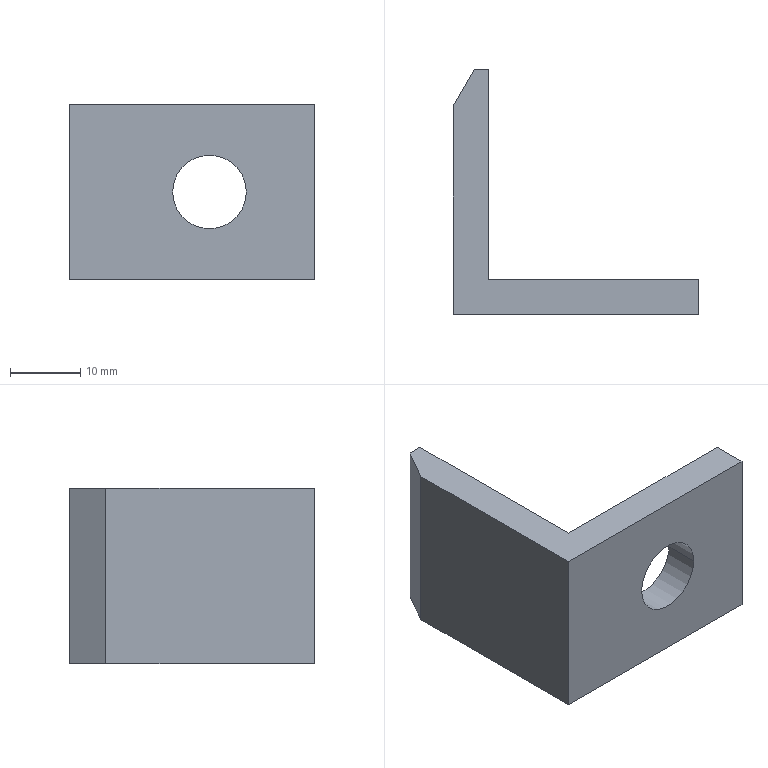Part | STEP file | 44-02-25 Lower Ejector Guide Plate | 1 solid | 11 faces | box 35 x 35 x 25 mm | volume 7497 mm3 | plane 9 | cylinder 2 | commonest cylinder face diameters 10.5 x2
STEP:
#1=CARTESIAN_POINT('',(0.,0.,0.));
#2=DIRECTION('',(0.,0.,1.));
#3=DIRECTION('',(1.,0.,0.));
#4=AXIS2_PLACEMENT_3D('',#1,#2,#3);
#5=CARTESIAN_POINT('',(14.75,0.,0.));
#6=VERTEX_POINT('',#5);
#7=CARTESIAN_POINT('',(14.75,5.,0.));
#8=VERTEX_POINT('',#7);
#9=CARTESIAN_POINT('',(14.75,0.,0.));
#10=DIRECTION('',(0.,1.,0.));
#11=VECTOR('',#10,1.);
#12=LINE('',#9,#11);
#13=CARTESIAN_POINT('',(20.,0.,0.));
#14=DIRECTION('',(0.,1.,0.));
#15=DIRECTION('',(-1.,0.,0.));
#16=AXIS2_PLACEMENT_3D('',#13,#14,#15);
#17=CYLINDRICAL_SURFACE('',#16,5.25);
#18=CARTESIAN_POINT('',(6.283,0.));
#19=DIRECTION('',(0.,1.));
#20=VECTOR('',#19,1.);
#21=LINE('',#18,#20);
#22=(GEOMETRIC_REPRESENTATION_CONTEXT(2)PARAMETRIC_REPRESENTATION_CONTEXT()REPRESENTATION_CONTEXT('',''));
#23=DEFINITIONAL_REPRESENTATION('',(#21),#22);
#24=PCURVE('',#17,#23);
#25=CARTESIAN_POINT('',(20.,0.,0.));
#26=DIRECTION('',(0.,1.,0.));
#27=DIRECTION('',(-1.,0.,0.));
#28=AXIS2_PLACEMENT_3D('',#25,#26,#27);
#29=CYLINDRICAL_SURFACE('',#28,5.25);
#30=CARTESIAN_POINT('',(0.,0.));
#31=DIRECTION('',(0.,1.));
#32=VECTOR('',#31,1.);
#33=LINE('',#30,#32);
#34=(GEOMETRIC_REPRESENTATION_CONTEXT(2)PARAMETRIC_REPRESENTATION_CONTEXT()REPRESENTATION_CONTEXT('',''));
#35=DEFINITIONAL_REPRESENTATION('',(#33),#34);
#36=PCURVE('',#29,#35);
#37=SURFACE_CURVE('',#12,(#24,#36),.PCURVE_S1.);
#38=EDGE_CURVE('',#6,#8,#37,.T.);
#39=ORIENTED_EDGE('',*,*,#38,.T.);
#40=CARTESIAN_POINT('',(25.25,5.,0.));
#41=VERTEX_POINT('',#40);
#42=CARTESIAN_POINT('',(20.,5.,0.));
#43=DIRECTION('',(0.,1.,0.));
#44=DIRECTION('',(-1.,0.,0.));
#45=AXIS2_PLACEMENT_3D('',#42,#43,#44);
#46=CIRCLE('',#45,5.25);
#47=CARTESIAN_POINT('',(0.,5.));
#48=DIRECTION('',(1.,0.));
#49=VECTOR('',#48,1.);
#50=LINE('',#47,#49);
#51=(GEOMETRIC_REPRESENTATION_CONTEXT(2)PARAMETRIC_REPRESENTATION_CONTEXT()REPRESENTATION_CONTEXT('',''));
#52=DEFINITIONAL_REPRESENTATION('',(#50),#51);
#53=PCURVE('',#17,#52);
#54=CARTESIAN_POINT('',(35.,5.,12.5));
#55=DIRECTION('',(0.,-1.,0.));
#56=DIRECTION('',(1.,0.,0.));
#57=AXIS2_PLACEMENT_3D('',#54,#55,#56);
#58=PLANE('',#57);
#59=CARTESIAN_POINT('',(-20.25,-12.5));
#60=CARTESIAN_POINT('',(-20.25,-3.407));
#61=CARTESIAN_POINT('',(-12.375,-7.953));
#62=CARTESIAN_POINT('',(-4.5,-12.5));
#63=CARTESIAN_POINT('',(-12.375,-17.047));
#64=CARTESIAN_POINT('',(-20.25,-21.593));
#65=CARTESIAN_POINT('',(-20.25,-12.5));
#66=(BOUNDED_CURVE()B_SPLINE_CURVE(2,(#59,#60,#61,#62,#63,#64,#65),.UNSPECIFIED.,.T.,.F.)B_SPLINE_CURVE_WITH_KNOTS((1,2,2,2,2,1),(-2.094,0.,2.094,4.189,6.283,8.378),.UNSPECIFIED.)CURVE()GEOMETRIC_REPRESENTATION_ITEM()RATIONAL_B_SPLINE_CURVE((1.,0.5,1.,0.5,1.,0.5,1.))REPRESENTATION_ITEM(''));
#67=(GEOMETRIC_REPRESENTATION_CONTEXT(2)PARAMETRIC_REPRESENTATION_CONTEXT()REPRESENTATION_CONTEXT('',''));
#68=DEFINITIONAL_REPRESENTATION('',(#66),#67);
#69=PCURVE('',#58,#68);
#70=SURFACE_CURVE('',#46,(#53,#69),.PCURVE_S1.);
#71=EDGE_CURVE('',#41,#8,#70,.T.);
#72=ORIENTED_EDGE('',*,*,#71,.F.);
#73=CARTESIAN_POINT('',(25.25,0.,0.));
#74=VERTEX_POINT('',#73);
#75=CARTESIAN_POINT('',(25.25,0.,0.));
#76=DIRECTION('',(0.,1.,0.));
#77=VECTOR('',#76,1.);
#78=LINE('',#75,#77);
#79=CARTESIAN_POINT('',(3.142,0.));
#80=DIRECTION('',(0.,1.));
#81=VECTOR('',#80,1.);
#82=LINE('',#79,#81);
#83=(GEOMETRIC_REPRESENTATION_CONTEXT(2)PARAMETRIC_REPRESENTATION_CONTEXT()REPRESENTATION_CONTEXT('',''));
#84=DEFINITIONAL_REPRESENTATION('',(#82),#83);
#85=PCURVE('',#17,#84);
#86=CARTESIAN_POINT('',(3.142,0.));
#87=DIRECTION('',(0.,1.));
#88=VECTOR('',#87,1.);
#89=LINE('',#86,#88);
#90=(GEOMETRIC_REPRESENTATION_CONTEXT(2)PARAMETRIC_REPRESENTATION_CONTEXT()REPRESENTATION_CONTEXT('',''));
#91=DEFINITIONAL_REPRESENTATION('',(#89),#90);
#92=PCURVE('',#29,#91);
#93=SURFACE_CURVE('',#78,(#85,#92),.PCURVE_S1.);
#94=EDGE_CURVE('',#74,#41,#93,.T.);
#95=ORIENTED_EDGE('',*,*,#94,.F.);
#96=CARTESIAN_POINT('',(20.,0.,0.));
#97=DIRECTION('',(0.,1.,0.));
#98=DIRECTION('',(-1.,0.,0.));
#99=AXIS2_PLACEMENT_3D('',#96,#97,#98);
#100=CIRCLE('',#99,5.25);
#101=CARTESIAN_POINT('',(0.,0.));
#102=DIRECTION('',(1.,0.));
#103=VECTOR('',#102,1.);
#104=LINE('',#101,#103);
#105=(GEOMETRIC_REPRESENTATION_CONTEXT(2)PARAMETRIC_REPRESENTATION_CONTEXT()REPRESENTATION_CONTEXT('',''));
#106=DEFINITIONAL_REPRESENTATION('',(#104),#105);
#107=PCURVE('',#17,#106);
#108=CARTESIAN_POINT('',(0.,0.,12.5));
#109=DIRECTION('',(0.,1.,0.));
#110=DIRECTION('',(0.,0.,1.));
#111=AXIS2_PLACEMENT_3D('',#108,#109,#110);
#112=PLANE('',#111);
#113=CARTESIAN_POINT('',(-12.5,20.));
#114=DIRECTION('',(0.,-1.));
#115=AXIS2_PLACEMENT_2D('',#113,#114);
#116=CIRCLE('',#115,5.25);
#117=(GEOMETRIC_REPRESENTATION_CONTEXT(2)PARAMETRIC_REPRESENTATION_CONTEXT()REPRESENTATION_CONTEXT('',''));
#118=DEFINITIONAL_REPRESENTATION('',(#116),#117);
#119=PCURVE('',#112,#118);
#120=SURFACE_CURVE('',#100,(#107,#119),.PCURVE_S1.);
#121=EDGE_CURVE('',#74,#6,#120,.T.);
#122=ORIENTED_EDGE('',*,*,#121,.T.);
#123=EDGE_LOOP('',(#39,#72,#95,#122));
#124=FACE_BOUND('',#123,.F.);
#125=ADVANCED_FACE('',(#124),#17,.F.);
#126=CARTESIAN_POINT('',(5.,35.,-12.5));
#127=VERTEX_POINT('',#126);
#128=CARTESIAN_POINT('',(3.,35.,-12.5));
#129=VERTEX_POINT('',#128);
#130=CARTESIAN_POINT('',(5.,35.,-12.5));
#131=DIRECTION('',(-1.,0.,0.));
#132=VECTOR('',#131,1.);
#133=LINE('',#130,#132);
#134=CARTESIAN_POINT('',(5.,35.,12.5));
#135=DIRECTION('',(0.,-1.,0.));
#136=DIRECTION('',(0.,0.,-1.));
#137=AXIS2_PLACEMENT_3D('',#134,#135,#136);
#138=PLANE('',#137);
#139=CARTESIAN_POINT('',(25.,0.));
#140=DIRECTION('',(0.,-1.));
#141=VECTOR('',#140,1.);
#142=LINE('',#139,#141);
#143=(GEOMETRIC_REPRESENTATION_CONTEXT(2)PARAMETRIC_REPRESENTATION_CONTEXT()REPRESENTATION_CONTEXT('',''));
#144=DEFINITIONAL_REPRESENTATION('',(#142),#143);
#145=PCURVE('',#138,#144);
#146=CARTESIAN_POINT('',(0.,0.,-12.5));
#147=DIRECTION('',(0.,0.,1.));
#148=DIRECTION('',(1.,0.,0.));
#149=AXIS2_PLACEMENT_3D('',#146,#147,#148);
#150=PLANE('',#149);
#151=CARTESIAN_POINT('',(5.,35.));
#152=DIRECTION('',(-1.,0.));
#153=VECTOR('',#152,1.);
#154=LINE('',#151,#153);
#155=(GEOMETRIC_REPRESENTATION_CONTEXT(2)PARAMETRIC_REPRESENTATION_CONTEXT()REPRESENTATION_CONTEXT('',''));
#156=DEFINITIONAL_REPRESENTATION('',(#154),#155);
#157=PCURVE('',#150,#156);
#158=SURFACE_CURVE('',#133,(#145,#157),.PCURVE_S1.);
#159=EDGE_CURVE('',#127,#129,#158,.T.);
#160=ORIENTED_EDGE('',*,*,#159,.T.);
#161=CARTESIAN_POINT('',(3.,35.,12.5));
#162=VERTEX_POINT('',#161);
#163=CARTESIAN_POINT('',(3.,35.,12.5));
#164=DIRECTION('',(0.,0.,1.));
#165=VECTOR('',#164,1.);
#166=LINE('',#163,#165);
#167=CARTESIAN_POINT('',(0.,-2.));
#168=DIRECTION('',(-1.,0.));
#169=VECTOR('',#168,1.);
#170=LINE('',#167,#169);
#171=(GEOMETRIC_REPRESENTATION_CONTEXT(2)PARAMETRIC_REPRESENTATION_CONTEXT()REPRESENTATION_CONTEXT('',''));
#172=DEFINITIONAL_REPRESENTATION('',(#170),#171);
#173=PCURVE('',#138,#172);
#174=CARTESIAN_POINT('',(0.,29.804,12.5));
#175=DIRECTION('',(0.866,-0.5,0.));
#176=DIRECTION('',(0.,0.,-1.));
#177=AXIS2_PLACEMENT_3D('',#174,#175,#176);
#178=PLANE('',#177);
#179=CARTESIAN_POINT('',(0.,6.));
#180=DIRECTION('',(-1.,0.));
#181=VECTOR('',#180,1.);
#182=LINE('',#179,#181);
#183=(GEOMETRIC_REPRESENTATION_CONTEXT(2)PARAMETRIC_REPRESENTATION_CONTEXT()REPRESENTATION_CONTEXT('',''));
#184=DEFINITIONAL_REPRESENTATION('',(#182),#183);
#185=PCURVE('',#178,#184);
#186=SURFACE_CURVE('',#166,(#173,#185),.PCURVE_S1.);
#187=EDGE_CURVE('',#129,#162,#186,.T.);
#188=ORIENTED_EDGE('',*,*,#187,.T.);
#189=CARTESIAN_POINT('',(5.,35.,12.5));
#190=VERTEX_POINT('',#189);
#191=CARTESIAN_POINT('',(5.,35.,12.5));
#192=DIRECTION('',(-1.,0.,0.));
#193=VECTOR('',#192,1.);
#194=LINE('',#191,#193);
#195=CARTESIAN_POINT('',(0.,0.));
#196=DIRECTION('',(0.,-1.));
#197=VECTOR('',#196,1.);
#198=LINE('',#195,#197);
#199=(GEOMETRIC_REPRESENTATION_CONTEXT(2)PARAMETRIC_REPRESENTATION_CONTEXT()REPRESENTATION_CONTEXT('',''));
#200=DEFINITIONAL_REPRESENTATION('',(#198),#199);
#201=PCURVE('',#138,#200);
#202=CARTESIAN_POINT('',(0.,0.,12.5));
#203=DIRECTION('',(0.,0.,1.));
#204=DIRECTION('',(1.,0.,0.));
#205=AXIS2_PLACEMENT_3D('',#202,#203,#204);
#206=PLANE('',#205);
#207=CARTESIAN_POINT('',(5.,35.));
#208=DIRECTION('',(-1.,0.));
#209=VECTOR('',#208,1.);
#210=LINE('',#207,#209);
#211=(GEOMETRIC_REPRESENTATION_CONTEXT(2)PARAMETRIC_REPRESENTATION_CONTEXT()REPRESENTATION_CONTEXT('',''));
#212=DEFINITIONAL_REPRESENTATION('',(#210),#211);
#213=PCURVE('',#206,#212);
#214=SURFACE_CURVE('',#194,(#201,#213),.PCURVE_S1.);
#215=EDGE_CURVE('',#190,#162,#214,.T.);
#216=ORIENTED_EDGE('',*,*,#215,.F.);
#217=CARTESIAN_POINT('',(5.,35.,12.5));
#218=DIRECTION('',(0.,0.,-1.));
#219=VECTOR('',#218,1.);
#220=LINE('',#217,#219);
#221=CARTESIAN_POINT('',(0.,0.));
#222=DIRECTION('',(1.,0.));
#223=VECTOR('',#222,1.);
#224=LINE('',#221,#223);
#225=(GEOMETRIC_REPRESENTATION_CONTEXT(2)PARAMETRIC_REPRESENTATION_CONTEXT()REPRESENTATION_CONTEXT('',''));
#226=DEFINITIONAL_REPRESENTATION('',(#224),#225);
#227=PCURVE('',#138,#226);
#228=CARTESIAN_POINT('',(5.,5.,12.5));
#229=DIRECTION('',(-1.,0.,0.));
#230=DIRECTION('',(0.,-1.,0.));
#231=AXIS2_PLACEMENT_3D('',#228,#229,#230);
#232=PLANE('',#231);
#233=CARTESIAN_POINT('',(-30.,0.));
#234=DIRECTION('',(0.,-1.));
#235=VECTOR('',#234,1.);
#236=LINE('',#233,#235);
#237=(GEOMETRIC_REPRESENTATION_CONTEXT(2)PARAMETRIC_REPRESENTATION_CONTEXT()REPRESENTATION_CONTEXT('',''));
#238=DEFINITIONAL_REPRESENTATION('',(#236),#237);
#239=PCURVE('',#232,#238);
#240=SURFACE_CURVE('',#220,(#227,#239),.PCURVE_S1.);
#241=EDGE_CURVE('',#190,#127,#240,.T.);
#242=ORIENTED_EDGE('',*,*,#241,.T.);
#243=EDGE_LOOP('',(#160,#188,#216,#242));
#244=FACE_BOUND('',#243,.T.);
#245=ADVANCED_FACE('',(#244),#138,.F.);
#246=CARTESIAN_POINT('',(0.,29.804,12.5));
#247=VERTEX_POINT('',#246);
#248=CARTESIAN_POINT('',(0.,0.,12.5));
#249=VERTEX_POINT('',#248);
#250=CARTESIAN_POINT('',(0.,35.,12.5));
#251=DIRECTION('',(0.,-1.,0.));
#252=VECTOR('',#251,1.);
#253=LINE('',#250,#252);
#254=CARTESIAN_POINT('',(0.,35.,12.5));
#255=DIRECTION('',(1.,0.,0.));
#256=DIRECTION('',(0.,0.,-1.));
#257=AXIS2_PLACEMENT_3D('',#254,#255,#256);
#258=PLANE('',#257);
#259=CARTESIAN_POINT('',(0.,0.));
#260=DIRECTION('',(0.,-1.));
#261=VECTOR('',#260,1.);
#262=LINE('',#259,#261);
#263=(GEOMETRIC_REPRESENTATION_CONTEXT(2)PARAMETRIC_REPRESENTATION_CONTEXT()REPRESENTATION_CONTEXT('',''));
#264=DEFINITIONAL_REPRESENTATION('',(#262),#263);
#265=PCURVE('',#258,#264);
#266=CARTESIAN_POINT('',(0.,35.));
#267=DIRECTION('',(0.,-1.));
#268=VECTOR('',#267,1.);
#269=LINE('',#266,#268);
#270=(GEOMETRIC_REPRESENTATION_CONTEXT(2)PARAMETRIC_REPRESENTATION_CONTEXT()REPRESENTATION_CONTEXT('',''));
#271=DEFINITIONAL_REPRESENTATION('',(#269),#270);
#272=PCURVE('',#206,#271);
#273=SURFACE_CURVE('',#253,(#265,#272),.PCURVE_S1.);
#274=EDGE_CURVE('',#247,#249,#273,.T.);
#275=ORIENTED_EDGE('',*,*,#274,.F.);
#276=CARTESIAN_POINT('',(0.,29.804,-12.5));
#277=VERTEX_POINT('',#276);
#278=CARTESIAN_POINT('',(0.,29.804,12.5));
#279=DIRECTION('',(0.,0.,-1.));
#280=VECTOR('',#279,1.);
#281=LINE('',#278,#280);
#282=CARTESIAN_POINT('',(0.,-5.196));
#283=DIRECTION('',(1.,0.));
#284=VECTOR('',#283,1.);
#285=LINE('',#282,#284);
#286=(GEOMETRIC_REPRESENTATION_CONTEXT(2)PARAMETRIC_REPRESENTATION_CONTEXT()REPRESENTATION_CONTEXT('',''));
#287=DEFINITIONAL_REPRESENTATION('',(#285),#286);
#288=PCURVE('',#258,#287);
#289=CARTESIAN_POINT('',(0.,0.));
#290=DIRECTION('',(1.,0.));
#291=VECTOR('',#290,1.);
#292=LINE('',#289,#291);
#293=(GEOMETRIC_REPRESENTATION_CONTEXT(2)PARAMETRIC_REPRESENTATION_CONTEXT()REPRESENTATION_CONTEXT('',''));
#294=DEFINITIONAL_REPRESENTATION('',(#292),#293);
#295=PCURVE('',#178,#294);
#296=SURFACE_CURVE('',#281,(#288,#295),.PCURVE_S1.);
#297=EDGE_CURVE('',#247,#277,#296,.T.);
#298=ORIENTED_EDGE('',*,*,#297,.T.);
#299=CARTESIAN_POINT('',(0.,0.,-12.5));
#300=VERTEX_POINT('',#299);
#301=CARTESIAN_POINT('',(0.,35.,-12.5));
#302=DIRECTION('',(0.,-1.,0.));
#303=VECTOR('',#302,1.);
#304=LINE('',#301,#303);
#305=CARTESIAN_POINT('',(25.,0.));
#306=DIRECTION('',(0.,-1.));
#307=VECTOR('',#306,1.);
#308=LINE('',#305,#307);
#309=(GEOMETRIC_REPRESENTATION_CONTEXT(2)PARAMETRIC_REPRESENTATION_CONTEXT()REPRESENTATION_CONTEXT('',''));
#310=DEFINITIONAL_REPRESENTATION('',(#308),#309);
#311=PCURVE('',#258,#310);
#312=CARTESIAN_POINT('',(0.,35.));
#313=DIRECTION('',(0.,-1.));
#314=VECTOR('',#313,1.);
#315=LINE('',#312,#314);
#316=(GEOMETRIC_REPRESENTATION_CONTEXT(2)PARAMETRIC_REPRESENTATION_CONTEXT()REPRESENTATION_CONTEXT('',''));
#317=DEFINITIONAL_REPRESENTATION('',(#315),#316);
#318=PCURVE('',#150,#317);
#319=SURFACE_CURVE('',#304,(#311,#318),.PCURVE_S1.);
#320=EDGE_CURVE('',#277,#300,#319,.T.);
#321=ORIENTED_EDGE('',*,*,#320,.T.);
#322=CARTESIAN_POINT('',(0.,0.,12.5));
#323=DIRECTION('',(0.,0.,-1.));
#324=VECTOR('',#323,1.);
#325=LINE('',#322,#324);
#326=CARTESIAN_POINT('',(0.,-35.));
#327=DIRECTION('',(1.,0.));
#328=VECTOR('',#327,1.);
#329=LINE('',#326,#328);
#330=(GEOMETRIC_REPRESENTATION_CONTEXT(2)PARAMETRIC_REPRESENTATION_CONTEXT()REPRESENTATION_CONTEXT('',''));
#331=DEFINITIONAL_REPRESENTATION('',(#329),#330);
#332=PCURVE('',#258,#331);
#333=CARTESIAN_POINT('',(0.,0.));
#334=DIRECTION('',(-1.,0.));
#335=VECTOR('',#334,1.);
#336=LINE('',#333,#335);
#337=(GEOMETRIC_REPRESENTATION_CONTEXT(2)PARAMETRIC_REPRESENTATION_CONTEXT()REPRESENTATION_CONTEXT('',''));
#338=DEFINITIONAL_REPRESENTATION('',(#336),#337);
#339=PCURVE('',#112,#338);
#340=SURFACE_CURVE('',#325,(#332,#339),.PCURVE_S1.);
#341=EDGE_CURVE('',#249,#300,#340,.T.);
#342=ORIENTED_EDGE('',*,*,#341,.F.);
#343=EDGE_LOOP('',(#275,#298,#321,#342));
#344=FACE_BOUND('',#343,.T.);
#345=ADVANCED_FACE('',(#344),#258,.F.);
#346=CARTESIAN_POINT('',(20.,0.,0.));
#347=DIRECTION('',(0.,1.,0.));
#348=DIRECTION('',(-1.,0.,0.));
#349=AXIS2_PLACEMENT_3D('',#346,#347,#348);
#350=CIRCLE('',#349,5.25);
#351=CARTESIAN_POINT('',(-12.5,20.));
#352=DIRECTION('',(0.,-1.));
#353=AXIS2_PLACEMENT_2D('',#351,#352);
#354=CIRCLE('',#353,5.25);
#355=(GEOMETRIC_REPRESENTATION_CONTEXT(2)PARAMETRIC_REPRESENTATION_CONTEXT()REPRESENTATION_CONTEXT('',''));
#356=DEFINITIONAL_REPRESENTATION('',(#354),#355);
#357=PCURVE('',#112,#356);
#358=CARTESIAN_POINT('',(0.,0.));
#359=DIRECTION('',(1.,0.));
#360=VECTOR('',#359,1.);
#361=LINE('',#358,#360);
#362=(GEOMETRIC_REPRESENTATION_CONTEXT(2)PARAMETRIC_REPRESENTATION_CONTEXT()REPRESENTATION_CONTEXT('',''));
#363=DEFINITIONAL_REPRESENTATION('',(#361),#362);
#364=PCURVE('',#29,#363);
#365=SURFACE_CURVE('',#350,(#357,#364),.PCURVE_S1.);
#366=EDGE_CURVE('',#6,#74,#365,.T.);
#367=ORIENTED_EDGE('',*,*,#366,.T.);
#368=ORIENTED_EDGE('',*,*,#121,.T.);
#369=EDGE_LOOP('',(#367,#368));
#370=FACE_BOUND('',#369,.T.);
#371=CARTESIAN_POINT('',(35.,0.,-12.5));
#372=VERTEX_POINT('',#371);
#373=CARTESIAN_POINT('',(0.,0.,-12.5));
#374=DIRECTION('',(1.,0.,0.));
#375=VECTOR('',#374,1.);
#376=LINE('',#373,#375);
#377=CARTESIAN_POINT('',(-25.,0.));
#378=DIRECTION('',(0.,1.));
#379=VECTOR('',#378,1.);
#380=LINE('',#377,#379);
#381=(GEOMETRIC_REPRESENTATION_CONTEXT(2)PARAMETRIC_REPRESENTATION_CONTEXT()REPRESENTATION_CONTEXT('',''));
#382=DEFINITIONAL_REPRESENTATION('',(#380),#381);
#383=PCURVE('',#112,#382);
#384=CARTESIAN_POINT('',(0.,0.));
#385=DIRECTION('',(1.,0.));
#386=VECTOR('',#385,1.);
#387=LINE('',#384,#386);
#388=(GEOMETRIC_REPRESENTATION_CONTEXT(2)PARAMETRIC_REPRESENTATION_CONTEXT()REPRESENTATION_CONTEXT('',''));
#389=DEFINITIONAL_REPRESENTATION('',(#387),#388);
#390=PCURVE('',#150,#389);
#391=SURFACE_CURVE('',#376,(#383,#390),.PCURVE_S1.);
#392=EDGE_CURVE('',#300,#372,#391,.T.);
#393=ORIENTED_EDGE('',*,*,#392,.T.);
#394=CARTESIAN_POINT('',(35.,0.,12.5));
#395=VERTEX_POINT('',#394);
#396=CARTESIAN_POINT('',(35.,0.,12.5));
#397=DIRECTION('',(0.,0.,-1.));
#398=VECTOR('',#397,1.);
#399=LINE('',#396,#398);
#400=CARTESIAN_POINT('',(0.,35.));
#401=DIRECTION('',(-1.,0.));
#402=VECTOR('',#401,1.);
#403=LINE('',#400,#402);
#404=(GEOMETRIC_REPRESENTATION_CONTEXT(2)PARAMETRIC_REPRESENTATION_CONTEXT()REPRESENTATION_CONTEXT('',''));
#405=DEFINITIONAL_REPRESENTATION('',(#403),#404);
#406=PCURVE('',#112,#405);
#407=CARTESIAN_POINT('',(35.,0.,12.5));
#408=DIRECTION('',(-1.,0.,0.));
#409=DIRECTION('',(0.,0.,1.));
#410=AXIS2_PLACEMENT_3D('',#407,#408,#409);
#411=PLANE('',#410);
#412=CARTESIAN_POINT('',(0.,0.));
#413=DIRECTION('',(-1.,0.));
#414=VECTOR('',#413,1.);
#415=LINE('',#412,#414);
#416=(GEOMETRIC_REPRESENTATION_CONTEXT(2)PARAMETRIC_REPRESENTATION_CONTEXT()REPRESENTATION_CONTEXT('',''));
#417=DEFINITIONAL_REPRESENTATION('',(#415),#416);
#418=PCURVE('',#411,#417);
#419=SURFACE_CURVE('',#399,(#406,#418),.PCURVE_S1.);
#420=EDGE_CURVE('',#395,#372,#419,.T.);
#421=ORIENTED_EDGE('',*,*,#420,.F.);
#422=CARTESIAN_POINT('',(0.,0.,12.5));
#423=DIRECTION('',(1.,0.,0.));
#424=VECTOR('',#423,1.);
#425=LINE('',#422,#424);
#426=CARTESIAN_POINT('',(0.,0.));
#427=DIRECTION('',(0.,1.));
#428=VECTOR('',#427,1.);
#429=LINE('',#426,#428);
#430=(GEOMETRIC_REPRESENTATION_CONTEXT(2)PARAMETRIC_REPRESENTATION_CONTEXT()REPRESENTATION_CONTEXT('',''));
#431=DEFINITIONAL_REPRESENTATION('',(#429),#430);
#432=PCURVE('',#112,#431);
#433=CARTESIAN_POINT('',(0.,0.));
#434=DIRECTION('',(1.,0.));
#435=VECTOR('',#434,1.);
#436=LINE('',#433,#435);
#437=(GEOMETRIC_REPRESENTATION_CONTEXT(2)PARAMETRIC_REPRESENTATION_CONTEXT()REPRESENTATION_CONTEXT('',''));
#438=DEFINITIONAL_REPRESENTATION('',(#436),#437);
#439=PCURVE('',#206,#438);
#440=SURFACE_CURVE('',#425,(#432,#439),.PCURVE_S1.);
#441=EDGE_CURVE('',#249,#395,#440,.T.);
#442=ORIENTED_EDGE('',*,*,#441,.F.);
#443=ORIENTED_EDGE('',*,*,#341,.T.);
#444=EDGE_LOOP('',(#393,#421,#442,#443));
#445=FACE_BOUND('',#444,.T.);
#446=ADVANCED_FACE('',(#370,#445),#112,.F.);
#447=CARTESIAN_POINT('',(35.,5.,-12.5));
#448=VERTEX_POINT('',#447);
#449=CARTESIAN_POINT('',(35.,0.,-12.5));
#450=DIRECTION('',(0.,1.,0.));
#451=VECTOR('',#450,1.);
#452=LINE('',#449,#451);
#453=CARTESIAN_POINT('',(-25.,0.));
#454=DIRECTION('',(0.,1.));
#455=VECTOR('',#454,1.);
#456=LINE('',#453,#455);
#457=(GEOMETRIC_REPRESENTATION_CONTEXT(2)PARAMETRIC_REPRESENTATION_CONTEXT()REPRESENTATION_CONTEXT('',''));
#458=DEFINITIONAL_REPRESENTATION('',(#456),#457);
#459=PCURVE('',#411,#458);
#460=CARTESIAN_POINT('',(35.,0.));
#461=DIRECTION('',(0.,1.));
#462=VECTOR('',#461,1.);
#463=LINE('',#460,#462);
#464=(GEOMETRIC_REPRESENTATION_CONTEXT(2)PARAMETRIC_REPRESENTATION_CONTEXT()REPRESENTATION_CONTEXT('',''));
#465=DEFINITIONAL_REPRESENTATION('',(#463),#464);
#466=PCURVE('',#150,#465);
#467=SURFACE_CURVE('',#452,(#459,#466),.PCURVE_S1.);
#468=EDGE_CURVE('',#372,#448,#467,.T.);
#469=ORIENTED_EDGE('',*,*,#468,.T.);
#470=CARTESIAN_POINT('',(35.,5.,12.5));
#471=VERTEX_POINT('',#470);
#472=CARTESIAN_POINT('',(35.,5.,12.5));
#473=DIRECTION('',(0.,0.,-1.));
#474=VECTOR('',#473,1.);
#475=LINE('',#472,#474);
#476=CARTESIAN_POINT('',(0.,5.));
#477=DIRECTION('',(-1.,0.));
#478=VECTOR('',#477,1.);
#479=LINE('',#476,#478);
#480=(GEOMETRIC_REPRESENTATION_CONTEXT(2)PARAMETRIC_REPRESENTATION_CONTEXT()REPRESENTATION_CONTEXT('',''));
#481=DEFINITIONAL_REPRESENTATION('',(#479),#480);
#482=PCURVE('',#411,#481);
#483=CARTESIAN_POINT('',(0.,0.));
#484=DIRECTION('',(0.,-1.));
#485=VECTOR('',#484,1.);
#486=LINE('',#483,#485);
#487=(GEOMETRIC_REPRESENTATION_CONTEXT(2)PARAMETRIC_REPRESENTATION_CONTEXT()REPRESENTATION_CONTEXT('',''));
#488=DEFINITIONAL_REPRESENTATION('',(#486),#487);
#489=PCURVE('',#58,#488);
#490=SURFACE_CURVE('',#475,(#482,#489),.PCURVE_S1.);
#491=EDGE_CURVE('',#471,#448,#490,.T.);
#492=ORIENTED_EDGE('',*,*,#491,.F.);
#493=CARTESIAN_POINT('',(35.,0.,12.5));
#494=DIRECTION('',(0.,1.,0.));
#495=VECTOR('',#494,1.);
#496=LINE('',#493,#495);
#497=CARTESIAN_POINT('',(0.,0.));
#498=DIRECTION('',(0.,1.));
#499=VECTOR('',#498,1.);
#500=LINE('',#497,#499);
#501=(GEOMETRIC_REPRESENTATION_CONTEXT(2)PARAMETRIC_REPRESENTATION_CONTEXT()REPRESENTATION_CONTEXT('',''));
#502=DEFINITIONAL_REPRESENTATION('',(#500),#501);
#503=PCURVE('',#411,#502);
#504=CARTESIAN_POINT('',(35.,0.));
#505=DIRECTION('',(0.,1.));
#506=VECTOR('',#505,1.);
#507=LINE('',#504,#506);
#508=(GEOMETRIC_REPRESENTATION_CONTEXT(2)PARAMETRIC_REPRESENTATION_CONTEXT()REPRESENTATION_CONTEXT('',''));
#509=DEFINITIONAL_REPRESENTATION('',(#507),#508);
#510=PCURVE('',#206,#509);
#511=SURFACE_CURVE('',#496,(#503,#510),.PCURVE_S1.);
#512=EDGE_CURVE('',#395,#471,#511,.T.);
#513=ORIENTED_EDGE('',*,*,#512,.F.);
#514=ORIENTED_EDGE('',*,*,#420,.T.);
#515=EDGE_LOOP('',(#469,#492,#513,#514));
#516=FACE_BOUND('',#515,.T.);
#517=ADVANCED_FACE('',(#516),#411,.F.);
#518=CARTESIAN_POINT('',(20.,5.,0.));
#519=DIRECTION('',(0.,1.,0.));
#520=DIRECTION('',(-1.,0.,0.));
#521=AXIS2_PLACEMENT_3D('',#518,#519,#520);
#522=CIRCLE('',#521,5.25);
#523=CARTESIAN_POINT('',(-20.25,-12.5));
#524=CARTESIAN_POINT('',(-20.25,-3.407));
#525=CARTESIAN_POINT('',(-12.375,-7.953));
#526=CARTESIAN_POINT('',(-4.5,-12.5));
#527=CARTESIAN_POINT('',(-12.375,-17.047));
#528=CARTESIAN_POINT('',(-20.25,-21.593));
#529=CARTESIAN_POINT('',(-20.25,-12.5));
#530=(BOUNDED_CURVE()B_SPLINE_CURVE(2,(#523,#524,#525,#526,#527,#528,#529),.UNSPECIFIED.,.T.,.F.)B_SPLINE_CURVE_WITH_KNOTS((1,2,2,2,2,1),(-2.094,0.,2.094,4.189,6.283,8.378),.UNSPECIFIED.)CURVE()GEOMETRIC_REPRESENTATION_ITEM()RATIONAL_B_SPLINE_CURVE((1.,0.5,1.,0.5,1.,0.5,1.))REPRESENTATION_ITEM(''));
#531=(GEOMETRIC_REPRESENTATION_CONTEXT(2)PARAMETRIC_REPRESENTATION_CONTEXT()REPRESENTATION_CONTEXT('',''));
#532=DEFINITIONAL_REPRESENTATION('',(#530),#531);
#533=PCURVE('',#58,#532);
#534=CARTESIAN_POINT('',(0.,5.));
#535=DIRECTION('',(1.,0.));
#536=VECTOR('',#535,1.);
#537=LINE('',#534,#536);
#538=(GEOMETRIC_REPRESENTATION_CONTEXT(2)PARAMETRIC_REPRESENTATION_CONTEXT()REPRESENTATION_CONTEXT('',''));
#539=DEFINITIONAL_REPRESENTATION('',(#537),#538);
#540=PCURVE('',#29,#539);
#541=SURFACE_CURVE('',#522,(#533,#540),.PCURVE_S1.);
#542=EDGE_CURVE('',#8,#41,#541,.T.);
#543=ORIENTED_EDGE('',*,*,#542,.F.);
#544=ORIENTED_EDGE('',*,*,#71,.F.);
#545=EDGE_LOOP('',(#543,#544));
#546=FACE_BOUND('',#545,.T.);
#547=CARTESIAN_POINT('',(5.,5.,-12.5));
#548=VERTEX_POINT('',#547);
#549=CARTESIAN_POINT('',(35.,5.,-12.5));
#550=DIRECTION('',(-1.,0.,0.));
#551=VECTOR('',#550,1.);
#552=LINE('',#549,#551);
#553=CARTESIAN_POINT('',(0.,-25.));
#554=DIRECTION('',(-1.,0.));
#555=VECTOR('',#554,1.);
#556=LINE('',#553,#555);
#557=(GEOMETRIC_REPRESENTATION_CONTEXT(2)PARAMETRIC_REPRESENTATION_CONTEXT()REPRESENTATION_CONTEXT('',''));
#558=DEFINITIONAL_REPRESENTATION('',(#556),#557);
#559=PCURVE('',#58,#558);
#560=CARTESIAN_POINT('',(35.,5.));
#561=DIRECTION('',(-1.,0.));
#562=VECTOR('',#561,1.);
#563=LINE('',#560,#562);
#564=(GEOMETRIC_REPRESENTATION_CONTEXT(2)PARAMETRIC_REPRESENTATION_CONTEXT()REPRESENTATION_CONTEXT('',''));
#565=DEFINITIONAL_REPRESENTATION('',(#563),#564);
#566=PCURVE('',#150,#565);
#567=SURFACE_CURVE('',#552,(#559,#566),.PCURVE_S1.);
#568=EDGE_CURVE('',#448,#548,#567,.T.);
#569=ORIENTED_EDGE('',*,*,#568,.T.);
#570=CARTESIAN_POINT('',(5.,5.,12.5));
#571=VERTEX_POINT('',#570);
#572=CARTESIAN_POINT('',(5.,5.,12.5));
#573=DIRECTION('',(0.,0.,-1.));
#574=VECTOR('',#573,1.);
#575=LINE('',#572,#574);
#576=CARTESIAN_POINT('',(-30.,0.));
#577=DIRECTION('',(0.,-1.));
#578=VECTOR('',#577,1.);
#579=LINE('',#576,#578);
#580=(GEOMETRIC_REPRESENTATION_CONTEXT(2)PARAMETRIC_REPRESENTATION_CONTEXT()REPRESENTATION_CONTEXT('',''));
#581=DEFINITIONAL_REPRESENTATION('',(#579),#580);
#582=PCURVE('',#58,#581);
#583=CARTESIAN_POINT('',(0.,0.));
#584=DIRECTION('',(0.,-1.));
#585=VECTOR('',#584,1.);
#586=LINE('',#583,#585);
#587=(GEOMETRIC_REPRESENTATION_CONTEXT(2)PARAMETRIC_REPRESENTATION_CONTEXT()REPRESENTATION_CONTEXT('',''));
#588=DEFINITIONAL_REPRESENTATION('',(#586),#587);
#589=PCURVE('',#232,#588);
#590=SURFACE_CURVE('',#575,(#582,#589),.PCURVE_S1.);
#591=EDGE_CURVE('',#571,#548,#590,.T.);
#592=ORIENTED_EDGE('',*,*,#591,.F.);
#593=CARTESIAN_POINT('',(35.,5.,12.5));
#594=DIRECTION('',(-1.,0.,0.));
#595=VECTOR('',#594,1.);
#596=LINE('',#593,#595);
#597=CARTESIAN_POINT('',(0.,0.));
#598=DIRECTION('',(-1.,0.));
#599=VECTOR('',#598,1.);
#600=LINE('',#597,#599);
#601=(GEOMETRIC_REPRESENTATION_CONTEXT(2)PARAMETRIC_REPRESENTATION_CONTEXT()REPRESENTATION_CONTEXT('',''));
#602=DEFINITIONAL_REPRESENTATION('',(#600),#601);
#603=PCURVE('',#58,#602);
#604=CARTESIAN_POINT('',(35.,5.));
#605=DIRECTION('',(-1.,0.));
#606=VECTOR('',#605,1.);
#607=LINE('',#604,#606);
#608=(GEOMETRIC_REPRESENTATION_CONTEXT(2)PARAMETRIC_REPRESENTATION_CONTEXT()REPRESENTATION_CONTEXT('',''));
#609=DEFINITIONAL_REPRESENTATION('',(#607),#608);
#610=PCURVE('',#206,#609);
#611=SURFACE_CURVE('',#596,(#603,#610),.PCURVE_S1.);
#612=EDGE_CURVE('',#471,#571,#611,.T.);
#613=ORIENTED_EDGE('',*,*,#612,.F.);
#614=ORIENTED_EDGE('',*,*,#491,.T.);
#615=EDGE_LOOP('',(#569,#592,#613,#614));
#616=FACE_BOUND('',#615,.T.);
#617=ADVANCED_FACE('',(#546,#616),#58,.F.);
#618=CARTESIAN_POINT('',(5.,5.,-12.5));
#619=DIRECTION('',(0.,1.,0.));
#620=VECTOR('',#619,1.);
#621=LINE('',#618,#620);
#622=CARTESIAN_POINT('',(0.,-25.));
#623=DIRECTION('',(-1.,0.));
#624=VECTOR('',#623,1.);
#625=LINE('',#622,#624);
#626=(GEOMETRIC_REPRESENTATION_CONTEXT(2)PARAMETRIC_REPRESENTATION_CONTEXT()REPRESENTATION_CONTEXT('',''));
#627=DEFINITIONAL_REPRESENTATION('',(#625),#626);
#628=PCURVE('',#232,#627);
#629=CARTESIAN_POINT('',(5.,5.));
#630=DIRECTION('',(0.,1.));
#631=VECTOR('',#630,1.);
#632=LINE('',#629,#631);
#633=(GEOMETRIC_REPRESENTATION_CONTEXT(2)PARAMETRIC_REPRESENTATION_CONTEXT()REPRESENTATION_CONTEXT('',''));
#634=DEFINITIONAL_REPRESENTATION('',(#632),#633);
#635=PCURVE('',#150,#634);
#636=SURFACE_CURVE('',#621,(#628,#635),.PCURVE_S1.);
#637=EDGE_CURVE('',#548,#127,#636,.T.);
#638=ORIENTED_EDGE('',*,*,#637,.T.);
#639=ORIENTED_EDGE('',*,*,#241,.F.);
#640=CARTESIAN_POINT('',(5.,5.,12.5));
#641=DIRECTION('',(0.,1.,0.));
#642=VECTOR('',#641,1.);
#643=LINE('',#640,#642);
#644=CARTESIAN_POINT('',(0.,0.));
#645=DIRECTION('',(-1.,0.));
#646=VECTOR('',#645,1.);
#647=LINE('',#644,#646);
#648=(GEOMETRIC_REPRESENTATION_CONTEXT(2)PARAMETRIC_REPRESENTATION_CONTEXT()REPRESENTATION_CONTEXT('',''));
#649=DEFINITIONAL_REPRESENTATION('',(#647),#648);
#650=PCURVE('',#232,#649);
#651=CARTESIAN_POINT('',(5.,5.));
#652=DIRECTION('',(0.,1.));
#653=VECTOR('',#652,1.);
#654=LINE('',#651,#653);
#655=(GEOMETRIC_REPRESENTATION_CONTEXT(2)PARAMETRIC_REPRESENTATION_CONTEXT()REPRESENTATION_CONTEXT('',''));
#656=DEFINITIONAL_REPRESENTATION('',(#654),#655);
#657=PCURVE('',#206,#656);
#658=SURFACE_CURVE('',#643,(#650,#657),.PCURVE_S1.);
#659=EDGE_CURVE('',#571,#190,#658,.T.);
#660=ORIENTED_EDGE('',*,*,#659,.F.);
#661=ORIENTED_EDGE('',*,*,#591,.T.);
#662=EDGE_LOOP('',(#638,#639,#660,#661));
#663=FACE_BOUND('',#662,.T.);
#664=ADVANCED_FACE('',(#663),#232,.F.);
#665=ORIENTED_EDGE('',*,*,#215,.T.);
#666=CARTESIAN_POINT('',(-12.905,7.451,12.5));
#667=DIRECTION('',(-0.5,-0.866,0.));
#668=VECTOR('',#667,1.);
#669=LINE('',#666,#668);
#670=CARTESIAN_POINT('',(-12.905,7.451));
#671=DIRECTION('',(-0.5,-0.866));
#672=VECTOR('',#671,1.);
#673=LINE('',#670,#672);
#674=(GEOMETRIC_REPRESENTATION_CONTEXT(2)PARAMETRIC_REPRESENTATION_CONTEXT()REPRESENTATION_CONTEXT('',''));
#675=DEFINITIONAL_REPRESENTATION('',(#673),#674);
#676=PCURVE('',#206,#675);
#677=CARTESIAN_POINT('',(0.,-25.811));
#678=DIRECTION('',(0.,-1.));
#679=VECTOR('',#678,1.);
#680=LINE('',#677,#679);
#681=(GEOMETRIC_REPRESENTATION_CONTEXT(2)PARAMETRIC_REPRESENTATION_CONTEXT()REPRESENTATION_CONTEXT('',''));
#682=DEFINITIONAL_REPRESENTATION('',(#680),#681);
#683=PCURVE('',#178,#682);
#684=SURFACE_CURVE('',#669,(#676,#683),.PCURVE_S1.);
#685=EDGE_CURVE('',#162,#247,#684,.T.);
#686=ORIENTED_EDGE('',*,*,#685,.T.);
#687=ORIENTED_EDGE('',*,*,#274,.T.);
#688=ORIENTED_EDGE('',*,*,#441,.T.);
#689=ORIENTED_EDGE('',*,*,#512,.T.);
#690=ORIENTED_EDGE('',*,*,#612,.T.);
#691=ORIENTED_EDGE('',*,*,#659,.T.);
#692=EDGE_LOOP('',(#665,#686,#687,#688,#689,#690,#691));
#693=FACE_BOUND('',#692,.T.);
#694=ADVANCED_FACE('',(#693),#206,.T.);
#695=ORIENTED_EDGE('',*,*,#320,.F.);
#696=CARTESIAN_POINT('',(0.,29.804,-12.5));
#697=DIRECTION('',(0.5,0.866,0.));
#698=VECTOR('',#697,1.);
#699=LINE('',#696,#698);
#700=CARTESIAN_POINT('',(0.,29.804));
#701=DIRECTION('',(0.5,0.866));
#702=VECTOR('',#701,1.);
#703=LINE('',#700,#702);
#704=(GEOMETRIC_REPRESENTATION_CONTEXT(2)PARAMETRIC_REPRESENTATION_CONTEXT()REPRESENTATION_CONTEXT('',''));
#705=DEFINITIONAL_REPRESENTATION('',(#703),#704);
#706=PCURVE('',#150,#705);
#707=CARTESIAN_POINT('',(25.,0.));
#708=DIRECTION('',(0.,1.));
#709=VECTOR('',#708,1.);
#710=LINE('',#707,#709);
#711=(GEOMETRIC_REPRESENTATION_CONTEXT(2)PARAMETRIC_REPRESENTATION_CONTEXT()REPRESENTATION_CONTEXT('',''));
#712=DEFINITIONAL_REPRESENTATION('',(#710),#711);
#713=PCURVE('',#178,#712);
#714=SURFACE_CURVE('',#699,(#706,#713),.PCURVE_S1.);
#715=EDGE_CURVE('',#277,#129,#714,.T.);
#716=ORIENTED_EDGE('',*,*,#715,.T.);
#717=ORIENTED_EDGE('',*,*,#159,.F.);
#718=ORIENTED_EDGE('',*,*,#637,.F.);
#719=ORIENTED_EDGE('',*,*,#568,.F.);
#720=ORIENTED_EDGE('',*,*,#468,.F.);
#721=ORIENTED_EDGE('',*,*,#392,.F.);
#722=EDGE_LOOP('',(#695,#716,#717,#718,#719,#720,#721));
#723=FACE_BOUND('',#722,.T.);
#724=ADVANCED_FACE('',(#723),#150,.F.);
#725=ORIENTED_EDGE('',*,*,#542,.F.);
#726=ORIENTED_EDGE('',*,*,#38,.F.);
#727=ORIENTED_EDGE('',*,*,#366,.T.);
#728=ORIENTED_EDGE('',*,*,#94,.T.);
#729=EDGE_LOOP('',(#725,#726,#727,#728));
#730=FACE_BOUND('',#729,.F.);
#731=ADVANCED_FACE('',(#730),#29,.F.);
#732=ORIENTED_EDGE('',*,*,#685,.F.);
#733=ORIENTED_EDGE('',*,*,#187,.F.);
#734=ORIENTED_EDGE('',*,*,#715,.F.);
#735=ORIENTED_EDGE('',*,*,#297,.F.);
#736=EDGE_LOOP('',(#732,#733,#734,#735));
#737=FACE_BOUND('',#736,.T.);
#738=ADVANCED_FACE('',(#737),#178,.F.);
#739=CLOSED_SHELL('',(#125,#245,#345,#446,#517,#617,#664,#694,#724,#731,#738));
#740=MANIFOLD_SOLID_BREP('',#739);
#741=(LENGTH_UNIT()NAMED_UNIT(*)SI_UNIT(.MILLI.,.METRE.));
#742=UNCERTAINTY_MEASURE_WITH_UNIT(LENGTH_MEASURE(0.0000001),#741,'','');
#743=(NAMED_UNIT(*)PLANE_ANGLE_UNIT()SI_UNIT($,.RADIAN.));
#744=(NAMED_UNIT(*)SI_UNIT($,.STERADIAN.)SOLID_ANGLE_UNIT());
#745=(GEOMETRIC_REPRESENTATION_CONTEXT(3)GLOBAL_UNCERTAINTY_ASSIGNED_CONTEXT((#742))GLOBAL_UNIT_ASSIGNED_CONTEXT((#741,#743,#744))REPRESENTATION_CONTEXT('',''));
#746=ADVANCED_BREP_SHAPE_REPRESENTATION('',(#4,#740),#745);